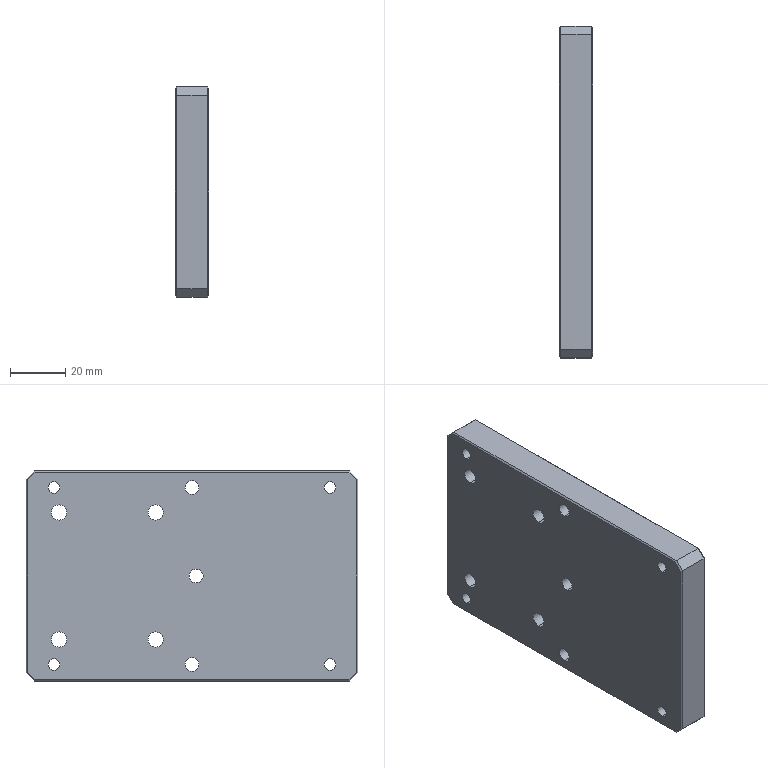Part | STEP file | HJDX-003 | 1 solid | 60 faces | box 12 x 120 x 76 mm | volume 105432 mm3 | cylinder 30 | plane 30 | commonest cylinder face diameters 4.2 x8 5.5 x8 10 x8 5 x6